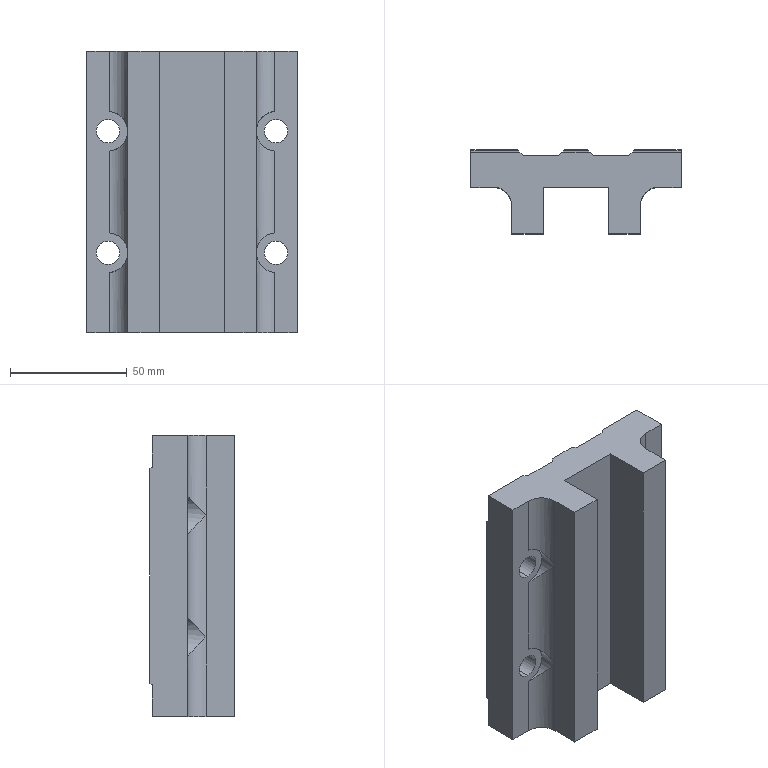Part | STEP file | P-008108 | 1 solid | 68 faces | box 90 x 36 x 120.4 mm | volume 224180 mm3 | plane 40 | cylinder 20 | cone 8 | commonest cylinder face diameters 10 x8 16 x6 17 x6